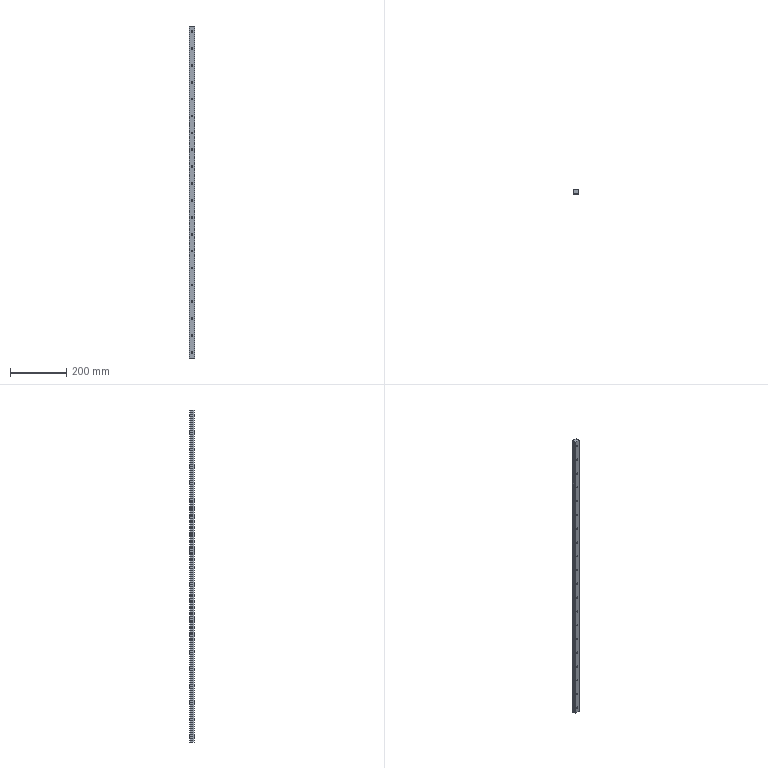Part | SolidWorks | features BaseBody 1 | 1 solid | 115 faces | box 20 x 15.5 x 1180 mm | volume 324435 mm3 | cylinder 85 | plane 30 | commonest cylinder face diameters 6 x40 9.5 x40 5 x3 3 x2